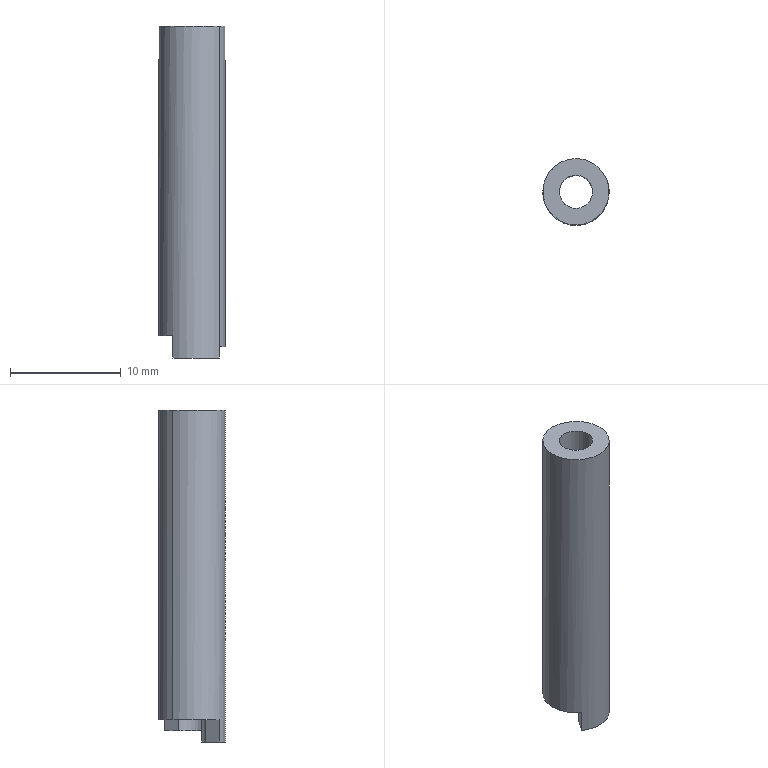Part | SolidWorks | features BaseBody 1 | 1 solid | 11 faces | box 6 x 6 x 30 mm | volume 609.259 mm3 | plane 7 | cylinder 4 | commonest cylinder face diameters 3.003 x2 6 x2
STEP:
#1=CARTESIAN_POINT('',(-75.39,-9.847,54.6));
#2=VERTEX_POINT('',#1);
#3=CARTESIAN_POINT('',(-75.758,-7.756,54.6));
#4=VERTEX_POINT('',#3);
#5=CARTESIAN_POINT('',(-74.528,-8.617,54.6));
#6=DIRECTION('',(0.,0.,-1.));
#7=DIRECTION('',(0.8192,-0.5736,0.));
#8=AXIS2_PLACEMENT_3D('',#5,#6,#7);
#9=CIRCLE('',#8,1.502);
#10=EDGE_CURVE('',#2,#4,#9,.T.);
#11=ORIENTED_EDGE('',*,*,#10,.T.);
#12=CARTESIAN_POINT('',(-75.758,-7.756,82.6));
#13=VERTEX_POINT('',#12);
#14=CARTESIAN_POINT('',(-75.758,-7.756,52.6));
#15=DIRECTION('',(0.,0.,1.));
#16=VECTOR('',#15,1000.);
#17=LINE('',#14,#16);
#18=EDGE_CURVE('',#4,#13,#17,.T.);
#19=ORIENTED_EDGE('',*,*,#18,.T.);
#20=CARTESIAN_POINT('',(-73.299,-9.478,82.6));
#21=VERTEX_POINT('',#20);
#22=CARTESIAN_POINT('',(-74.528,-8.617,82.6));
#23=DIRECTION('',(0.,0.,-1.));
#24=DIRECTION('',(0.8192,-0.5736,0.));
#25=AXIS2_PLACEMENT_3D('',#22,#23,#24);
#26=CIRCLE('',#25,1.502);
#27=EDGE_CURVE('',#21,#13,#26,.T.);
#28=ORIENTED_EDGE('',*,*,#27,.F.);
#29=CARTESIAN_POINT('',(-73.299,-9.478,53.6));
#30=VERTEX_POINT('',#29);
#31=CARTESIAN_POINT('',(-73.299,-9.478,52.6));
#32=DIRECTION('',(0.,0.,1.));
#33=VECTOR('',#32,1000.);
#34=LINE('',#31,#33);
#35=EDGE_CURVE('',#30,#21,#34,.T.);
#36=ORIENTED_EDGE('',*,*,#35,.F.);
#37=CARTESIAN_POINT('',(-73.299,-9.478,52.6));
#38=VERTEX_POINT('',#37);
#39=CARTESIAN_POINT('',(-73.299,-9.478,52.6));
#40=DIRECTION('',(0.,0.,-1.));
#41=VECTOR('',#40,1000.);
#42=LINE('',#39,#41);
#43=EDGE_CURVE('',#30,#38,#42,.T.);
#44=ORIENTED_EDGE('',*,*,#43,.T.);
#45=CARTESIAN_POINT('',(-75.39,-9.847,52.6));
#46=VERTEX_POINT('',#45);
#47=CARTESIAN_POINT('',(-74.528,-8.617,52.6));
#48=DIRECTION('',(0.,0.,1.));
#49=DIRECTION('',(0.8192,-0.5736,0.));
#50=AXIS2_PLACEMENT_3D('',#47,#48,#49);
#51=CIRCLE('',#50,1.502);
#52=EDGE_CURVE('',#46,#38,#51,.T.);
#53=ORIENTED_EDGE('',*,*,#52,.F.);
#54=CARTESIAN_POINT('',(-75.39,-9.847,52.6));
#55=DIRECTION('',(0.,0.,1.));
#56=VECTOR('',#55,1000.);
#57=LINE('',#54,#56);
#58=EDGE_CURVE('',#46,#2,#57,.T.);
#59=ORIENTED_EDGE('',*,*,#58,.T.);
#60=EDGE_LOOP('',(#11,#19,#28,#36,#44,#53,#59));
#61=FACE_OUTER_BOUND('',#60,.T.);
#62=CARTESIAN_POINT('',(-74.528,-8.617,52.6));
#63=DIRECTION('',(0.,0.,1.));
#64=DIRECTION('',(0.8192,-0.5736,0.));
#65=AXIS2_PLACEMENT_3D('',#62,#63,#64);
#66=CYLINDRICAL_SURFACE('',#65,1.502);
#67=ADVANCED_FACE('',(#61),#66,.F.);
#68=CARTESIAN_POINT('',(-76.986,-6.896,54.6));
#69=VERTEX_POINT('',#68);
#70=CARTESIAN_POINT('',(-72.808,-6.16,54.6));
#71=VERTEX_POINT('',#70);
#72=CARTESIAN_POINT('',(-74.528,-8.617,54.6));
#73=DIRECTION('',(0.,0.,-1.));
#74=DIRECTION('',(0.8192,-0.5736,0.));
#75=AXIS2_PLACEMENT_3D('',#72,#73,#74);
#76=CIRCLE('',#75,3.);
#77=EDGE_CURVE('',#69,#71,#76,.T.);
#78=ORIENTED_EDGE('',*,*,#77,.F.);
#79=CARTESIAN_POINT('',(-76.986,-6.896,82.6));
#80=VERTEX_POINT('',#79);
#81=CARTESIAN_POINT('',(-76.986,-6.896,52.6));
#82=DIRECTION('',(0.,0.,1.));
#83=VECTOR('',#82,1000.);
#84=LINE('',#81,#83);
#85=EDGE_CURVE('',#69,#80,#84,.T.);
#86=ORIENTED_EDGE('',*,*,#85,.T.);
#87=CARTESIAN_POINT('',(-72.071,-10.338,82.6));
#88=VERTEX_POINT('',#87);
#89=CARTESIAN_POINT('',(-74.528,-8.617,82.6));
#90=DIRECTION('',(0.,0.,-1.));
#91=DIRECTION('',(0.8192,-0.5736,0.));
#92=AXIS2_PLACEMENT_3D('',#89,#90,#91);
#93=CIRCLE('',#92,3.);
#94=EDGE_CURVE('',#80,#88,#93,.T.);
#95=ORIENTED_EDGE('',*,*,#94,.T.);
#96=CARTESIAN_POINT('',(-72.071,-10.338,53.6));
#97=VERTEX_POINT('',#96);
#98=CARTESIAN_POINT('',(-72.071,-10.338,52.6));
#99=DIRECTION('',(0.,0.,1.));
#100=VECTOR('',#99,1000.);
#101=LINE('',#98,#100);
#102=EDGE_CURVE('',#97,#88,#101,.T.);
#103=ORIENTED_EDGE('',*,*,#102,.F.);
#104=CARTESIAN_POINT('',(-72.808,-6.16,53.6));
#105=VERTEX_POINT('',#104);
#106=CARTESIAN_POINT('',(-74.528,-8.617,53.6));
#107=DIRECTION('',(0.,0.,-1.));
#108=DIRECTION('',(0.8192,-0.5736,0.));
#109=AXIS2_PLACEMENT_3D('',#106,#107,#108);
#110=CIRCLE('',#109,3.);
#111=EDGE_CURVE('',#105,#97,#110,.T.);
#112=ORIENTED_EDGE('',*,*,#111,.F.);
#113=CARTESIAN_POINT('',(-72.808,-6.16,52.6));
#114=DIRECTION('',(0.,0.,-1.));
#115=VECTOR('',#114,1000.);
#116=LINE('',#113,#115);
#117=EDGE_CURVE('',#71,#105,#116,.T.);
#118=ORIENTED_EDGE('',*,*,#117,.F.);
#119=EDGE_LOOP('',(#78,#86,#95,#103,#112,#118));
#120=FACE_OUTER_BOUND('',#119,.T.);
#121=CARTESIAN_POINT('',(-74.528,-8.617,52.6));
#122=DIRECTION('',(0.,0.,1.));
#123=DIRECTION('',(0.8192,-0.5736,0.));
#124=AXIS2_PLACEMENT_3D('',#121,#122,#123);
#125=CYLINDRICAL_SURFACE('',#124,3.);
#126=ADVANCED_FACE('',(#120),#125,.T.);
#127=ORIENTED_EDGE('',*,*,#27,.T.);
#128=CARTESIAN_POINT('',(-74.528,-8.617,82.6));
#129=DIRECTION('',(0.,0.,-1.));
#130=DIRECTION('',(0.8192,-0.5736,0.));
#131=AXIS2_PLACEMENT_3D('',#128,#129,#130);
#132=CIRCLE('',#131,1.502);
#133=EDGE_CURVE('',#13,#21,#132,.T.);
#134=ORIENTED_EDGE('',*,*,#133,.T.);
#135=EDGE_LOOP('',(#127,#134));
#136=FACE_BOUND('',#135,.T.);
#137=CARTESIAN_POINT('',(-74.528,-8.617,82.6));
#138=DIRECTION('',(0.,0.,-1.));
#139=DIRECTION('',(0.8192,-0.5736,0.));
#140=AXIS2_PLACEMENT_3D('',#137,#138,#139);
#141=CIRCLE('',#140,3.);
#142=EDGE_CURVE('',#88,#80,#141,.T.);
#143=ORIENTED_EDGE('',*,*,#142,.F.);
#144=ORIENTED_EDGE('',*,*,#94,.F.);
#145=EDGE_LOOP('',(#143,#144));
#146=FACE_OUTER_BOUND('',#145,.T.);
#147=CARTESIAN_POINT('',(-74.528,-8.617,82.6));
#148=DIRECTION('',(0.,0.,1.));
#149=DIRECTION('',(0.8192,-0.5736,0.));
#150=AXIS2_PLACEMENT_3D('',#147,#148,#149);
#151=PLANE('',#150);
#152=ADVANCED_FACE('',(#136,#146),#151,.T.);
#153=CARTESIAN_POINT('',(-72.071,-10.338,52.6));
#154=VERTEX_POINT('',#153);
#155=CARTESIAN_POINT('',(-74.528,-8.617,52.6));
#156=DIRECTION('',(0.8192,-0.5736,0.));
#157=VECTOR('',#156,1000.);
#158=LINE('',#155,#157);
#159=EDGE_CURVE('',#38,#154,#158,.T.);
#160=ORIENTED_EDGE('',*,*,#159,.T.);
#161=CARTESIAN_POINT('',(-76.249,-11.074,52.6));
#162=VERTEX_POINT('',#161);
#163=CARTESIAN_POINT('',(-74.528,-8.617,52.6));
#164=DIRECTION('',(0.,0.,1.));
#165=DIRECTION('',(0.8192,-0.5736,0.));
#166=AXIS2_PLACEMENT_3D('',#163,#164,#165);
#167=CIRCLE('',#166,3.);
#168=EDGE_CURVE('',#162,#154,#167,.T.);
#169=ORIENTED_EDGE('',*,*,#168,.F.);
#170=CARTESIAN_POINT('',(-74.528,-8.617,52.6));
#171=DIRECTION('',(0.5736,0.8192,0.));
#172=VECTOR('',#171,1000.);
#173=LINE('',#170,#172);
#174=EDGE_CURVE('',#162,#46,#173,.T.);
#175=ORIENTED_EDGE('',*,*,#174,.T.);
#176=ORIENTED_EDGE('',*,*,#52,.T.);
#177=EDGE_LOOP('',(#160,#169,#175,#176));
#178=FACE_OUTER_BOUND('',#177,.T.);
#179=CARTESIAN_POINT('',(-74.528,-8.617,52.6));
#180=DIRECTION('',(0.,0.,-1.));
#181=DIRECTION('',(-0.8192,0.5736,0.));
#182=AXIS2_PLACEMENT_3D('',#179,#180,#181);
#183=PLANE('',#182);
#184=ADVANCED_FACE('',(#178),#183,.T.);
#185=ORIENTED_EDGE('',*,*,#85,.F.);
#186=CARTESIAN_POINT('',(-76.249,-11.074,54.6));
#187=VERTEX_POINT('',#186);
#188=CARTESIAN_POINT('',(-74.528,-8.617,54.6));
#189=DIRECTION('',(0.,0.,-1.));
#190=DIRECTION('',(0.8192,-0.5736,0.));
#191=AXIS2_PLACEMENT_3D('',#188,#189,#190);
#192=CIRCLE('',#191,3.);
#193=EDGE_CURVE('',#187,#69,#192,.T.);
#194=ORIENTED_EDGE('',*,*,#193,.F.);
#195=CARTESIAN_POINT('',(-76.249,-11.074,52.6));
#196=DIRECTION('',(0.,0.,1.));
#197=VECTOR('',#196,1000.);
#198=LINE('',#195,#197);
#199=EDGE_CURVE('',#162,#187,#198,.T.);
#200=ORIENTED_EDGE('',*,*,#199,.F.);
#201=ORIENTED_EDGE('',*,*,#168,.T.);
#202=CARTESIAN_POINT('',(-72.071,-10.338,52.6));
#203=DIRECTION('',(0.,0.,-1.));
#204=VECTOR('',#203,1000.);
#205=LINE('',#202,#204);
#206=EDGE_CURVE('',#97,#154,#205,.T.);
#207=ORIENTED_EDGE('',*,*,#206,.F.);
#208=ORIENTED_EDGE('',*,*,#102,.T.);
#209=ORIENTED_EDGE('',*,*,#142,.T.);
#210=EDGE_LOOP('',(#185,#194,#200,#201,#207,#208,#209));
#211=FACE_OUTER_BOUND('',#210,.T.);
#212=CARTESIAN_POINT('',(-74.528,-8.617,52.6));
#213=DIRECTION('',(0.,0.,1.));
#214=DIRECTION('',(0.8192,-0.5736,0.));
#215=AXIS2_PLACEMENT_3D('',#212,#213,#214);
#216=CYLINDRICAL_SURFACE('',#215,3.);
#217=ADVANCED_FACE('',(#211),#216,.T.);
#218=ORIENTED_EDGE('',*,*,#18,.F.);
#219=CARTESIAN_POINT('',(-73.667,-7.387,54.6));
#220=VERTEX_POINT('',#219);
#221=CARTESIAN_POINT('',(-74.528,-8.617,54.6));
#222=DIRECTION('',(0.,0.,-1.));
#223=DIRECTION('',(0.8192,-0.5736,0.));
#224=AXIS2_PLACEMENT_3D('',#221,#222,#223);
#225=CIRCLE('',#224,1.502);
#226=EDGE_CURVE('',#4,#220,#225,.T.);
#227=ORIENTED_EDGE('',*,*,#226,.T.);
#228=CARTESIAN_POINT('',(-73.667,-7.387,53.6));
#229=VERTEX_POINT('',#228);
#230=CARTESIAN_POINT('',(-73.667,-7.387,52.6));
#231=DIRECTION('',(0.,0.,-1.));
#232=VECTOR('',#231,1000.);
#233=LINE('',#230,#232);
#234=EDGE_CURVE('',#220,#229,#233,.T.);
#235=ORIENTED_EDGE('',*,*,#234,.T.);
#236=CARTESIAN_POINT('',(-74.528,-8.617,53.6));
#237=DIRECTION('',(0.,0.,-1.));
#238=DIRECTION('',(0.8192,-0.5736,0.));
#239=AXIS2_PLACEMENT_3D('',#236,#237,#238);
#240=CIRCLE('',#239,1.501);
#241=EDGE_CURVE('',#229,#30,#240,.T.);
#242=ORIENTED_EDGE('',*,*,#241,.T.);
#243=ORIENTED_EDGE('',*,*,#35,.T.);
#244=ORIENTED_EDGE('',*,*,#133,.F.);
#245=EDGE_LOOP('',(#218,#227,#235,#242,#243,#244));
#246=FACE_OUTER_BOUND('',#245,.T.);
#247=CARTESIAN_POINT('',(-74.528,-8.617,52.6));
#248=DIRECTION('',(0.,0.,1.));
#249=DIRECTION('',(0.8192,-0.5736,0.));
#250=AXIS2_PLACEMENT_3D('',#247,#248,#249);
#251=CYLINDRICAL_SURFACE('',#250,1.502);
#252=ADVANCED_FACE('',(#246),#251,.F.);
#253=ORIENTED_EDGE('',*,*,#193,.T.);
#254=ORIENTED_EDGE('',*,*,#77,.T.);
#255=CARTESIAN_POINT('',(-74.528,-8.617,54.6));
#256=DIRECTION('',(0.5736,0.8192,0.));
#257=VECTOR('',#256,1000.);
#258=LINE('',#255,#257);
#259=EDGE_CURVE('',#220,#71,#258,.T.);
#260=ORIENTED_EDGE('',*,*,#259,.F.);
#261=ORIENTED_EDGE('',*,*,#226,.F.);
#262=ORIENTED_EDGE('',*,*,#10,.F.);
#263=CARTESIAN_POINT('',(-74.528,-8.617,54.6));
#264=DIRECTION('',(0.5736,0.8192,0.));
#265=VECTOR('',#264,1000.);
#266=LINE('',#263,#265);
#267=EDGE_CURVE('',#187,#2,#266,.T.);
#268=ORIENTED_EDGE('',*,*,#267,.F.);
#269=EDGE_LOOP('',(#253,#254,#260,#261,#262,#268));
#270=FACE_OUTER_BOUND('',#269,.T.);
#271=CARTESIAN_POINT('',(-76.168,-7.469,54.6));
#272=DIRECTION('',(0.,0.,1.));
#273=DIRECTION('',(-0.8192,0.5736,0.));
#274=AXIS2_PLACEMENT_3D('',#271,#272,#273);
#275=PLANE('',#274);
#276=ADVANCED_FACE('',(#270),#275,.F.);
#277=ORIENTED_EDGE('',*,*,#117,.T.);
#278=CARTESIAN_POINT('',(-74.528,-8.617,53.6));
#279=DIRECTION('',(-0.5736,-0.8192,0.));
#280=VECTOR('',#279,1000.);
#281=LINE('',#278,#280);
#282=EDGE_CURVE('',#105,#229,#281,.T.);
#283=ORIENTED_EDGE('',*,*,#282,.T.);
#284=ORIENTED_EDGE('',*,*,#234,.F.);
#285=ORIENTED_EDGE('',*,*,#259,.T.);
#286=EDGE_LOOP('',(#277,#283,#284,#285));
#287=FACE_OUTER_BOUND('',#286,.T.);
#288=CARTESIAN_POINT('',(-74.528,-8.617,54.6));
#289=DIRECTION('',(0.8192,-0.5736,0.));
#290=DIRECTION('',(0.,0.,1.));
#291=AXIS2_PLACEMENT_3D('',#288,#289,#290);
#292=PLANE('',#291);
#293=ADVANCED_FACE('',(#287),#292,.F.);
#294=ORIENTED_EDGE('',*,*,#199,.T.);
#295=ORIENTED_EDGE('',*,*,#267,.T.);
#296=ORIENTED_EDGE('',*,*,#58,.F.);
#297=ORIENTED_EDGE('',*,*,#174,.F.);
#298=EDGE_LOOP('',(#294,#295,#296,#297));
#299=FACE_OUTER_BOUND('',#298,.T.);
#300=CARTESIAN_POINT('',(-74.528,-8.617,54.6));
#301=DIRECTION('',(0.8192,-0.5736,0.));
#302=DIRECTION('',(0.,0.,1.));
#303=AXIS2_PLACEMENT_3D('',#300,#301,#302);
#304=PLANE('',#303);
#305=ADVANCED_FACE('',(#299),#304,.F.);
#306=ORIENTED_EDGE('',*,*,#206,.T.);
#307=ORIENTED_EDGE('',*,*,#159,.F.);
#308=ORIENTED_EDGE('',*,*,#43,.F.);
#309=CARTESIAN_POINT('',(-74.528,-8.617,53.6));
#310=DIRECTION('',(0.8192,-0.5736,0.));
#311=VECTOR('',#310,1000.);
#312=LINE('',#309,#311);
#313=EDGE_CURVE('',#30,#97,#312,.T.);
#314=ORIENTED_EDGE('',*,*,#313,.T.);
#315=EDGE_LOOP('',(#306,#307,#308,#314));
#316=FACE_OUTER_BOUND('',#315,.T.);
#317=CARTESIAN_POINT('',(-74.528,-8.617,53.6));
#318=DIRECTION('',(-0.5736,-0.8192,0.));
#319=DIRECTION('',(0.,0.,-1.));
#320=AXIS2_PLACEMENT_3D('',#317,#318,#319);
#321=PLANE('',#320);
#322=ADVANCED_FACE('',(#316),#321,.F.);
#323=ORIENTED_EDGE('',*,*,#111,.T.);
#324=ORIENTED_EDGE('',*,*,#313,.F.);
#325=ORIENTED_EDGE('',*,*,#241,.F.);
#326=ORIENTED_EDGE('',*,*,#282,.F.);
#327=EDGE_LOOP('',(#323,#324,#325,#326));
#328=FACE_OUTER_BOUND('',#327,.T.);
#329=CARTESIAN_POINT('',(-73.38,-6.977,53.6));
#330=DIRECTION('',(0.,0.,1.));
#331=DIRECTION('',(-0.8192,0.5736,0.));
#332=AXIS2_PLACEMENT_3D('',#329,#330,#331);
#333=PLANE('',#332);
#334=ADVANCED_FACE('',(#328),#333,.F.);
#335=CLOSED_SHELL('',(#67,#126,#152,#184,#217,#252,#276,#293,#305,#322,#334));
#336=MANIFOLD_SOLID_BREP('',#335);
#337=CARTESIAN_POINT('',(0.,0.,0.));
#338=DIRECTION('',(0.,0.,1.));
#339=DIRECTION('',(1.,0.,0.));
#340=AXIS2_PLACEMENT_3D('',#337,#338,#339);
#341=(LENGTH_UNIT()NAMED_UNIT(*)SI_UNIT(.MILLI.,.METRE.));
#342=UNCERTAINTY_MEASURE_WITH_UNIT(LENGTH_MEASURE(0.00001),#341,'','');
#343=(NAMED_UNIT(*)PLANE_ANGLE_UNIT()SI_UNIT($,.RADIAN.));
#344=(NAMED_UNIT(*)SI_UNIT($,.STERADIAN.)SOLID_ANGLE_UNIT());
#345=(GEOMETRIC_REPRESENTATION_CONTEXT(3)GLOBAL_UNCERTAINTY_ASSIGNED_CONTEXT((#342))GLOBAL_UNIT_ASSIGNED_CONTEXT((#341,#343,#344))REPRESENTATION_CONTEXT('',''));
#346=ADVANCED_BREP_SHAPE_REPRESENTATION('',(#336,#340),#345);